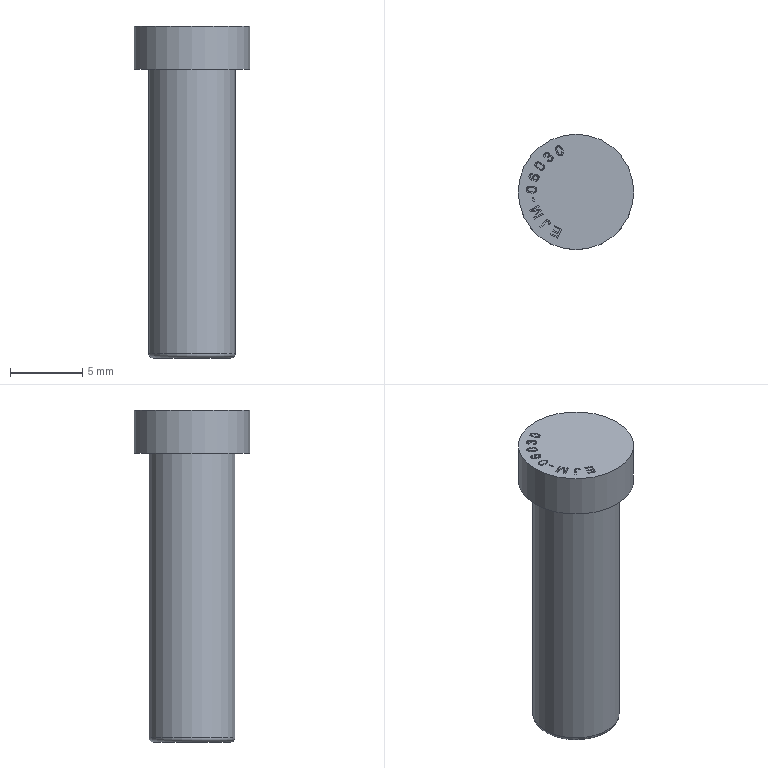Part | STEP file | lll_id2514_x_t | 1 solid | 81 faces | box 8 x 8 x 23 mm | volume 715.678 mm3 | plane 49 | other 29 | cylinder 2 | torus 1 | commonest cylinder face diameters 6 x1 8 x1